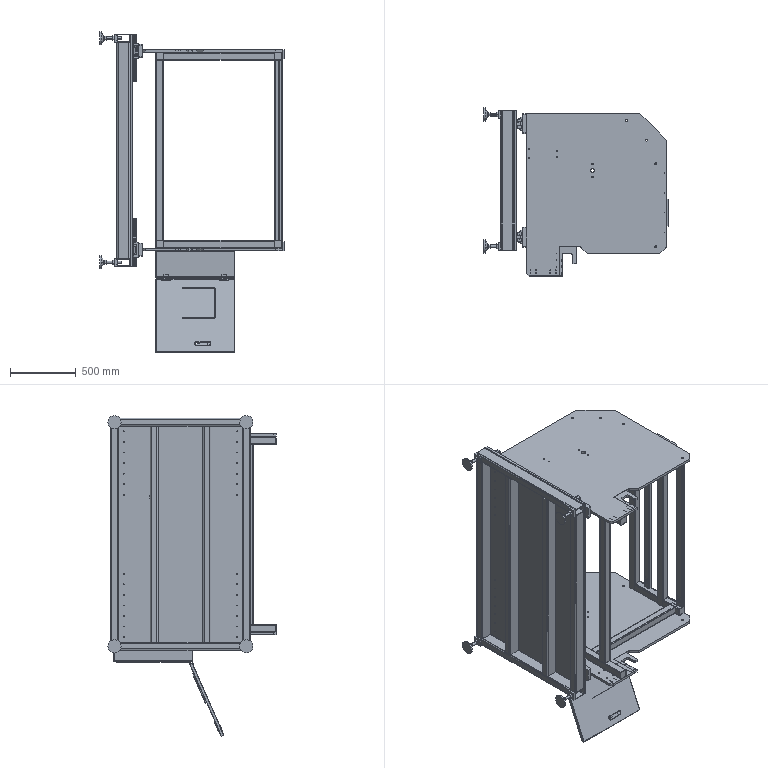Part | SolidWorks | features CompositeCurve 2 | 69 solids | 3427 faces | volume 105601898 mm3 | plane 2188 | cylinder 921 | spline 276 | cone 42 | commonest cylinder face diameters 6.8 x118 5 x106 10 x81 9 x58 6.4 x48 12.8 x48